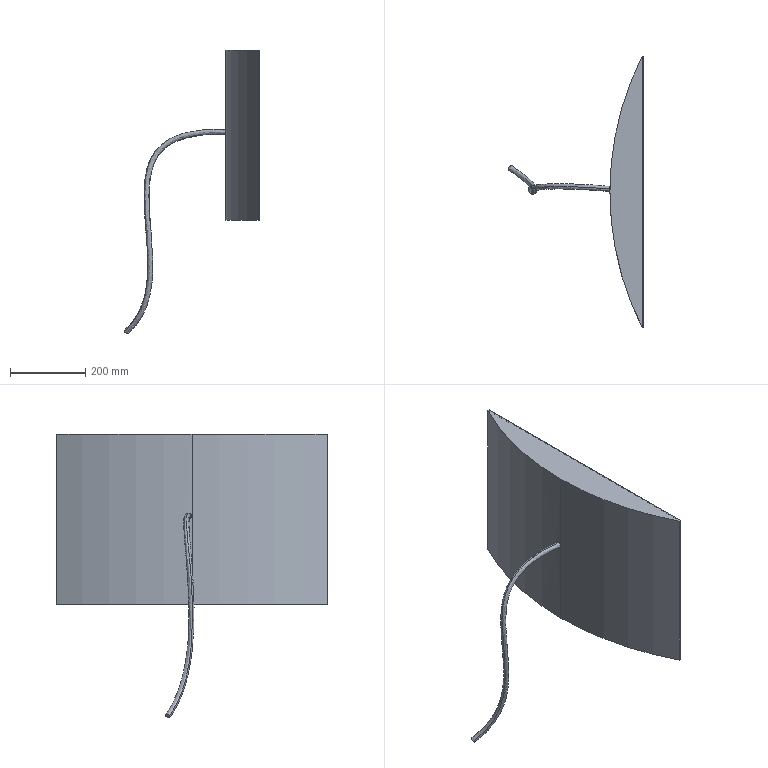Part | SolidWorks | features 3DProfileFeature 2, Extrusion 1, ICE 1, Sweep 1 | 1 solid | 15 faces | box 360.915 x 719 x 753.544 mm | volume 19467710 mm3 | plane 11 | spline 2 | cylinder 2 | commonest cylinder face diameters 1600 x2